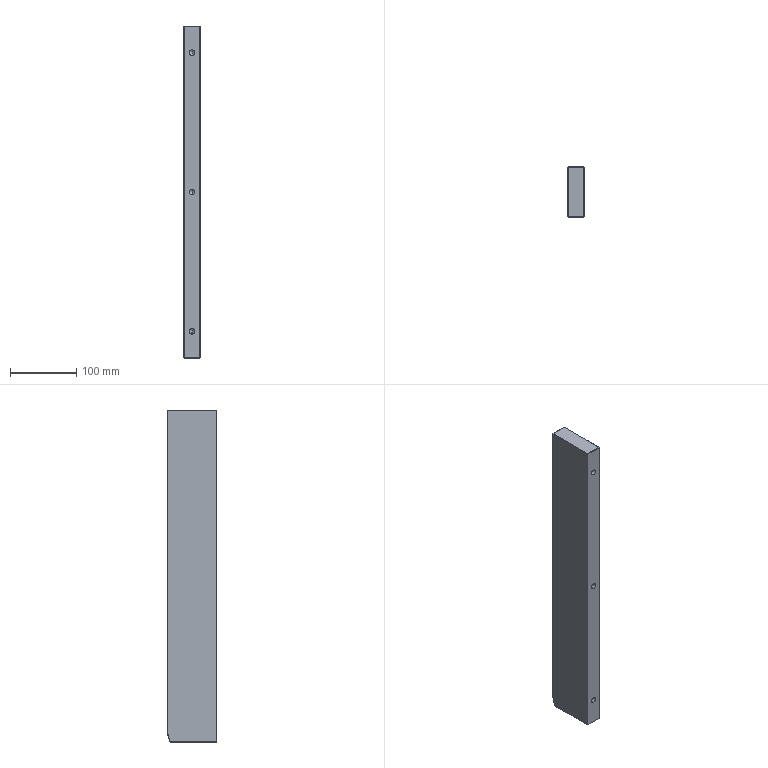Part | STEP file | OP10-019_base rib (B) | 1 solid | 49 faces | box 25 x 75 x 500 mm | volume 929254 mm3 | plane 29 | cylinder 10 | cone 10 | commonest cylinder face diameters 8.5 x10